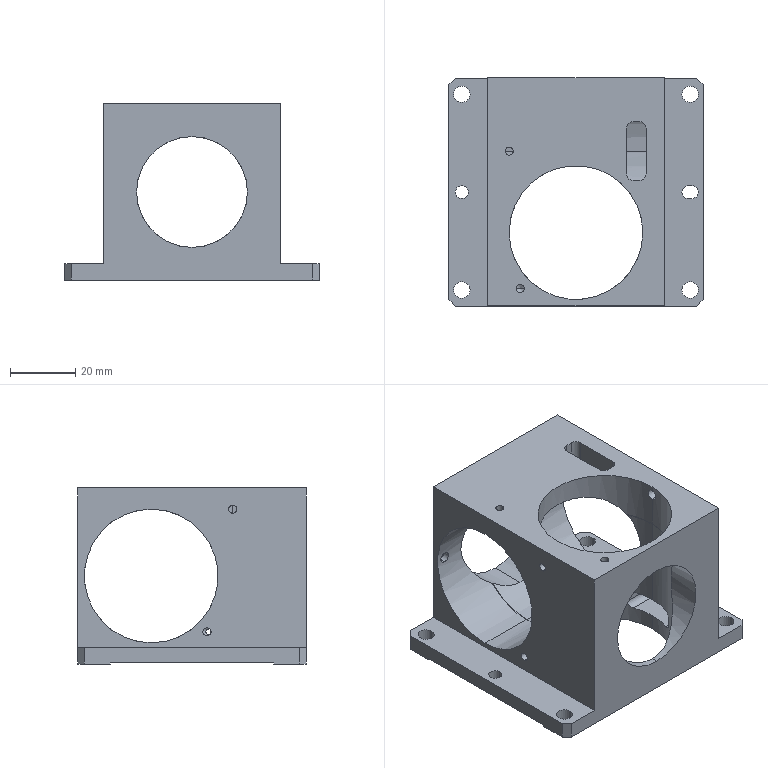NC program | NX | posted with a generic post | part box 78 x 70 x 54 mm
Whole program:
N10 G17 G21 G94 G90
(HOLE_MILLING_COPY_1 , TOOL : D20)
N12 T02 M6
N14 G54
N16 G17 G0 G90 X0. Y12.5 B0. C0. S9500 M3
N18 G43 Z30. H2
N20 Z-11.5
N22 G94 G3 X5.2 Y17.7 R5.2 F2000.
N24 X0. Y22.9 R5.2
N26 X0. Y22.9 Z-12. I0. J-10.4
N28 X0. Y22.9 Z-12.5 I0. J-10.4
N30 X0. Y22.9 Z-13. I0. J-10.4
N32 X0. Y22.9 Z-13.5 I0. J-10.4
N34 X0. Y22.9 Z-14. I0. J-10.4
N36 X0. Y22.9 Z-14.5 I0. J-10.4
N38 X0. Y22.9 Z-15. I0. J-10.4
N40 X0. Y22.9 Z-15.5 I0. J-10.4
N42 X0. Y22.9 Z-16. I0. J-10.4
N44 X0. Y22.9 Z-16.5 I0. J-10.4
N46 X0. Y22.9 Z-17. I0. J-10.4
N48 X0. Y22.9 Z-17.5 I0. J-10.4
N50 X0. Y22.9 Z-18. I0. J-10.4
N52 X0. Y22.9 Z-18.5 I0. J-10.4
N54 X0. Y22.9 Z-19. I0. J-10.4
N56 X0. Y22.9 Z-19.5 I0. J-10.4
N58 X0. Y22.9 Z-20. I0. J-10.4
N60 X0. Y22.9 Z-20.5 I0. J-10.4
N62 X0. Y22.9 Z-21. I0. J-10.4
N64 X0. Y22.9 Z-21.5 I0. J-10.4
N66 X0. Y22.9 Z-22. I0. J-10.4
N68 X0. Y22.9 Z-22.5 I0. J-10.4
N70 X0. Y22.9 Z-23. I0. J-10.4
N72 X0. Y22.9 Z-23.5 I0. J-10.4
N74 X0. Y22.9 Z-24. I0. J-10.4
N76 X0. Y22.9 Z-24.5 I0. J-10.4
N78 X0. Y22.9 Z-25. I0. J-10.4
N80 X0. Y22.9 Z-25.5 I0. J-10.4
N82 X0. Y22.9 Z-26. I0. J-10.4
N84 X0. Y22.9 Z-26.5 I0. J-10.4
N86 X0. Y22.9 Z-27. I0. J-10.4
N88 X0. Y22.9 Z-27.5 I0. J-10.4
N90 X0. Y22.9 Z-28. I0. J-10.4
N92 X0. Y22.9 Z-28.5 I0. J-10.4
N94 X0. Y22.9 Z-29. I0. J-10.4
N96 X0. Y22.9 Z-29.5 I0. J-10.4
N98 X0. Y22.9 Z-30. I0. J-10.4
N100 X0. Y22.9 Z-30.5 I0. J-10.4
N102 X0. Y22.9 Z-31. I0. J-10.4
N104 X0. Y22.9 Z-31.5 I0. J-10.4
N106 X0. Y22.9 Z-32. I0. J-10.4
N108 X0. Y22.9 Z-32.5 I0. J-10.4
N110 X0. Y22.9 Z-33. I0. J-10.4
N112 X0. Y22.9 Z-33.5 I0. J-10.4
N114 X0. Y22.9 Z-34. I0. J-10.4
N116 X0. Y22.9 Z-34.5 I0. J-10.4
N118 X0. Y22.9 Z-35. I0. J-10.4
N120 X0. Y22.9 Z-35.5 I0. J-10.4
N122 X0. Y22.9 Z-36. I0. J-10.4
N124 X0. Y22.9 Z-36.5 I0. J-10.4
N126 X0. Y22.9 Z-37. I0. J-10.4
N128 X0. Y22.9 Z-37.5 I0. J-10.4
N130 X0. Y22.9 Z-38. I0. J-10.4
N132 X0. Y22.9 Z-38.5 I0. J-10.4
N134 X0. Y22.9 Z-39. I0. J-10.4
N136 X0. Y22.9 Z-39.5 I0. J-10.4
N138 X0. Y22.9 Z-40. I0. J-10.4
N140 X0. Y22.9 Z-40.5 I0. J-10.4
N142 X0. Y22.9 Z-41. I0. J-10.4
N144 X0. Y22.9 Z-41.5 I0. J-10.4
N146 X0. Y22.9 Z-42. I0. J-10.4
N148 X0. Y22.9 Z-42.5 I0. J-10.4
N150 X0. Y22.9 Z-43. I0. J-10.4
N152 X0. Y22.9 Z-43.5 I0. J-10.4
N154 X0. Y22.9 Z-44. I0. J-10.4
N156 X0. Y22.9 Z-44.5 I0. J-10.4
N158 X0. Y22.9 Z-45. I0. J-10.4
N160 X0. Y22.9 Z-45.5 I0. J-10.4
N162 X0. Y22.9 Z-46. I0. J-10.4
N164 X0. Y22.9 Z-46.5 I0. J-10.4
N166 X0. Y22.9 Z-47. I0. J-10.4
N168 X0. Y22.9 Z-47.5 I0. J-10.4
N170 X0. Y22.9 Z-48. I0. J-10.4
N172 X0. Y22.9 Z-48.5 I0. J-10.4
N174 X0. Y22.9 Z-49. I0. J-10.4
N176 X0. Y22.9 Z-49.5 I0. J-10.4
N178 X0. Y22.9 Z-50. I0. J-10.4
N180 X0. Y22.9 Z-50.5 I0. J-10.4
N182 X0. Y22.9 Z-51. I0. J-10.4
N184 X0. Y22.9 Z-51.5 I0. J-10.4
N186 X0. Y22.9 Z-52. I0. J-10.4
N188 X0. Y22.9 Z-52.5 I0. J-10.4
N190 X0. Y22.9 Z-53. I0. J-10.4
N192 X0. Y22.9 Z-53.5 I0. J-10.4
N194 X0. Y22.9 Z-54. I0. J-10.4
N196 X0. Y22.9 Z-54.5 I0. J-10.4
N198 X0. Y22.9 Z-55. I0. J-10.4
N200 X0. Y22.9 Z-55.5 I0. J-10.4
N202 X0. Y22.9 Z-56. I0. J-10.4
N204 X0. Y22.9 Z-56.5 I0. J-10.4
N206 X0. Y22.9 Z-57. I0. J-10.4
N208 X0. Y22.9 Z-57.5 I0. J-10.4
N210 X0. Y22.9 Z-58. I0. J-10.4
N212 X0. Y22.9 Z-58.5 I0. J-10.4
N214 X0. Y22.9 Z-59. I0. J-10.4
N216 X0. Y22.9 Z-59.5 I0. J-10.4
N218 X0. Y22.9 Z-60. I0. J-10.4
N220 X0. Y22.9 Z-60.5 I0. J-10.4
N222 X0. Y22.9 Z-61. I0. J-10.4
N224 X0. Y22.9 Z-61.5 I0. J-10.4
N226 X0. Y22.9 Z-62. I0. J-10.4
N228 X0. Y22.9 Z-62.5 I0. J-10.4
N230 X0. Y22.9 Z-63. I0. J-10.4
N232 X0. Y22.9 Z-63.5 I0. J-10.4
N234 X0. Y22.9 Z-64. I0. J-10.4
N236 X0. Y22.9 Z-64.5 I0. J-10.4
N238 X0. Y22.9 Z-65. I0. J-10.4
N240 X0. Y22.9 Z-65.5 I0. J-10.4
N242 X0. Y22.9 Z-66. I0. J-10.4
N244 X-10.4 Y12.5 R10.4
N246 X0. Y22.9 R-10.4
N248 X-5.2 Y17.7 R5.2
N250 X0. Y12.5 R5.2
N252 G0 Z30.
N254 M5
(DRILLING_1_COPY_1_COPY_1 , TOOL : D6A45)
N256 T07 M6
N258 G54
N260 G17 G0 G90 X-17.1 Y-4.6 B0. C0. S5000 M3
N262 G43 Z30. H7
N264 G94 G81 G98 Z-13.5 F250. R-9.
N266 X20.5 Y-12.5
N268 G80
N270 G0 X20.5 Y-12.5 Z30.
N272 M5
(DRILLING_COPY_COPY , TOOL : 2.5ZT)
N274 T12 M6
N276 G54
N278 G17 G0 G90 X-17.1 Y-4.6 B0. C0. S2000 M3
N280 G43 Z30. H12
N282 G94 G83 G98 Z-20.251 F120. Q2. R-9.
N284 X20.5 Y-12.5 Z-20.789
N286 G80
N288 G0 X20.5 Y-12.5 Z30.
N290 M5
(PLANAR_MILL_COPY_1_1_COPY_COPY_1_COPY , TOOL : D6A45)
N292 T07 M6
N294 G54
N296 G17 G0 G90 X-17.3 Y7.296 B0. C0. S9500 M3
N298 G43 Z30. H7
N300 Z-11.5
N302 G94 G1 Z-13. F1250.
N304 X-18. Y6.892
N306 G3 X-18.5 Y6.026 R1.
N308 X-18.5 Y18.974 R-19.6
N310 X-18. Y18.108 R1.
N312 G1 X-17.3 Y17.704
N314 Z-11.5
N316 G0 Z30.
N318 M5
(TOOLCOMP_COPY , TOOL : D16JING)
N320 T13 M6
N322 G54
N324 G17 G0 G90 X0. Y12.5 B0. C0. S9500 M3
N326 G43 Z30. H13
N328 Z-11.5
N330 G41 G94 G1 X3.043 Y21.394 F1000. D13
N332 G3 X0. Y24.95 R3.08
N334 X0. Y24.95 Z-21.5 I0. J-12.45
N336 X0. Y24.95 Z-31.5 I0. J-12.45
N338 X0. Y24.95 Z-41.5 I0. J-12.45
N340 X0. Y24.95 Z-51.5 I0. J-12.45
N342 X0. Y24.95 Z-61.5 I0. J-12.45
N344 X-3.847 Y0.659 Z-66. R12.45
N346 X11.841 Y8.653 R12.45
N348 X-3.847 Y0.659 R-12.45
N350 X0.146 Y3.101 R3.08
N352 G40
N354 G1 X0. Y12.5
N356 G0 Z30.
N358 M5
N360 M2